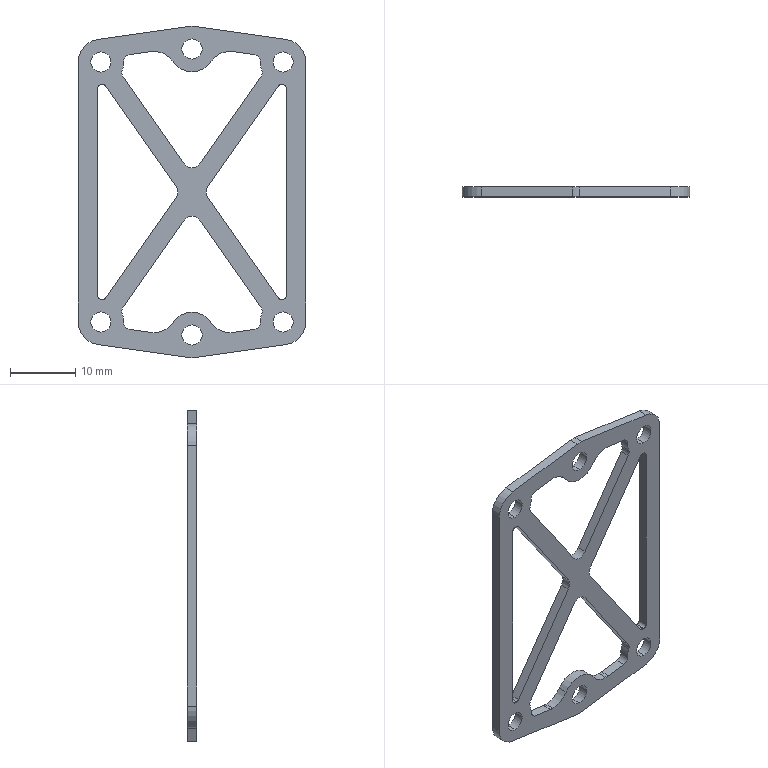Part | SolidWorks | features Fillet 4, Extrusion 1 | 1 solid | 81 faces | box 35 x 1.5 x 51 mm | volume 1129 mm3 | cylinder 59 | plane 22 | commonest cylinder face diameters 7 x24 3.1 x12 1 x10 2 x8 3 x5